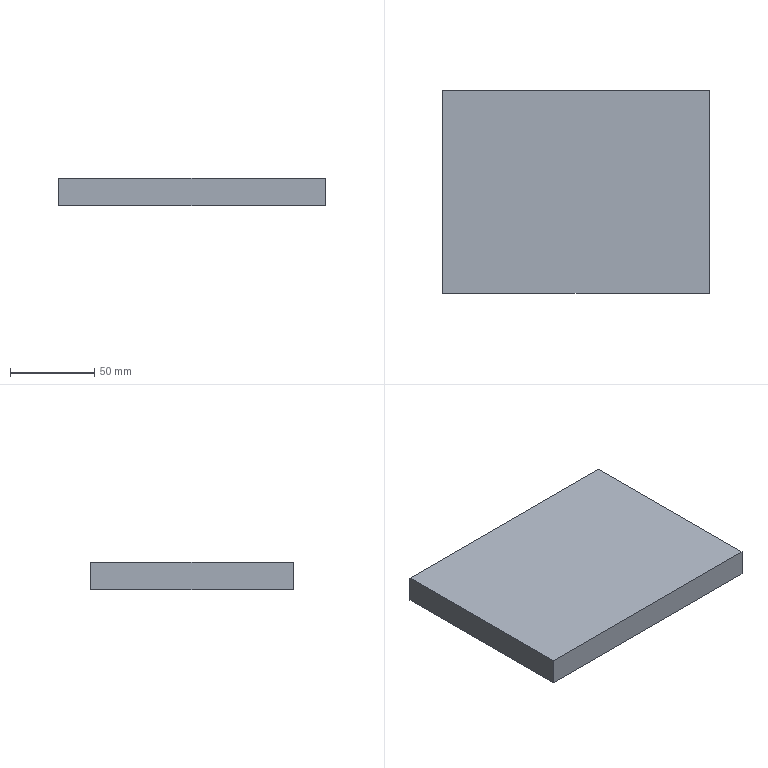Part | STEP file | 07-Square plate | 1 solid | 6 faces | box 158 x 120 x 16 mm | volume 303360 mm3 | plane 6
STEP:
#1=CARTESIAN_POINT('',(0.,0.,0.));
#2=DIRECTION('',(0.,0.,1.));
#3=DIRECTION('',(1.,0.,0.));
#4=AXIS2_PLACEMENT_3D('',#1,#2,#3);
#5=CARTESIAN_POINT('',(0.,0.,0.));
#6=VERTEX_POINT('',#5);
#7=CARTESIAN_POINT('',(0.,-120.,0.));
#8=VERTEX_POINT('',#7);
#9=CARTESIAN_POINT('',(0.,0.,0.));
#10=DIRECTION('',(0.,-1.,0.));
#11=VECTOR('',#10,1.);
#12=LINE('',#9,#11);
#13=CARTESIAN_POINT('',(0.,0.,16.));
#14=DIRECTION('',(1.,0.,0.));
#15=DIRECTION('',(0.,1.,0.));
#16=AXIS2_PLACEMENT_3D('',#13,#14,#15);
#17=PLANE('',#16);
#18=CARTESIAN_POINT('',(0.,-16.));
#19=DIRECTION('',(-1.,0.));
#20=VECTOR('',#19,1.);
#21=LINE('',#18,#20);
#22=(GEOMETRIC_REPRESENTATION_CONTEXT(2)PARAMETRIC_REPRESENTATION_CONTEXT()REPRESENTATION_CONTEXT('',''));
#23=DEFINITIONAL_REPRESENTATION('',(#21),#22);
#24=PCURVE('',#17,#23);
#25=CARTESIAN_POINT('',(0.,0.,0.));
#26=DIRECTION('',(0.,0.,1.));
#27=DIRECTION('',(1.,0.,0.));
#28=AXIS2_PLACEMENT_3D('',#25,#26,#27);
#29=PLANE('',#28);
#30=CARTESIAN_POINT('',(0.,0.));
#31=DIRECTION('',(0.,-1.));
#32=VECTOR('',#31,1.);
#33=LINE('',#30,#32);
#34=(GEOMETRIC_REPRESENTATION_CONTEXT(2)PARAMETRIC_REPRESENTATION_CONTEXT()REPRESENTATION_CONTEXT('',''));
#35=DEFINITIONAL_REPRESENTATION('',(#33),#34);
#36=PCURVE('',#29,#35);
#37=SURFACE_CURVE('',#12,(#24,#36),.PCURVE_S1.);
#38=EDGE_CURVE('',#6,#8,#37,.T.);
#39=ORIENTED_EDGE('',*,*,#38,.T.);
#40=CARTESIAN_POINT('',(0.,-120.,16.));
#41=VERTEX_POINT('',#40);
#42=CARTESIAN_POINT('',(0.,-120.,16.));
#43=DIRECTION('',(0.,0.,-1.));
#44=VECTOR('',#43,1.);
#45=LINE('',#42,#44);
#46=CARTESIAN_POINT('',(-120.,0.));
#47=DIRECTION('',(0.,-1.));
#48=VECTOR('',#47,1.);
#49=LINE('',#46,#48);
#50=(GEOMETRIC_REPRESENTATION_CONTEXT(2)PARAMETRIC_REPRESENTATION_CONTEXT()REPRESENTATION_CONTEXT('',''));
#51=DEFINITIONAL_REPRESENTATION('',(#49),#50);
#52=PCURVE('',#17,#51);
#53=CARTESIAN_POINT('',(0.,-120.,16.));
#54=DIRECTION('',(0.,1.,0.));
#55=DIRECTION('',(0.,0.,1.));
#56=AXIS2_PLACEMENT_3D('',#53,#54,#55);
#57=PLANE('',#56);
#58=CARTESIAN_POINT('',(0.,0.));
#59=DIRECTION('',(-1.,0.));
#60=VECTOR('',#59,1.);
#61=LINE('',#58,#60);
#62=(GEOMETRIC_REPRESENTATION_CONTEXT(2)PARAMETRIC_REPRESENTATION_CONTEXT()REPRESENTATION_CONTEXT('',''));
#63=DEFINITIONAL_REPRESENTATION('',(#61),#62);
#64=PCURVE('',#57,#63);
#65=SURFACE_CURVE('',#45,(#52,#64),.PCURVE_S1.);
#66=EDGE_CURVE('',#41,#8,#65,.T.);
#67=ORIENTED_EDGE('',*,*,#66,.F.);
#68=CARTESIAN_POINT('',(0.,0.,16.));
#69=VERTEX_POINT('',#68);
#70=CARTESIAN_POINT('',(0.,0.,16.));
#71=DIRECTION('',(0.,-1.,0.));
#72=VECTOR('',#71,1.);
#73=LINE('',#70,#72);
#74=CARTESIAN_POINT('',(0.,0.));
#75=DIRECTION('',(-1.,0.));
#76=VECTOR('',#75,1.);
#77=LINE('',#74,#76);
#78=(GEOMETRIC_REPRESENTATION_CONTEXT(2)PARAMETRIC_REPRESENTATION_CONTEXT()REPRESENTATION_CONTEXT('',''));
#79=DEFINITIONAL_REPRESENTATION('',(#77),#78);
#80=PCURVE('',#17,#79);
#81=CARTESIAN_POINT('',(0.,0.,16.));
#82=DIRECTION('',(0.,0.,1.));
#83=DIRECTION('',(1.,0.,0.));
#84=AXIS2_PLACEMENT_3D('',#81,#82,#83);
#85=PLANE('',#84);
#86=CARTESIAN_POINT('',(0.,0.));
#87=DIRECTION('',(0.,-1.));
#88=VECTOR('',#87,1.);
#89=LINE('',#86,#88);
#90=(GEOMETRIC_REPRESENTATION_CONTEXT(2)PARAMETRIC_REPRESENTATION_CONTEXT()REPRESENTATION_CONTEXT('',''));
#91=DEFINITIONAL_REPRESENTATION('',(#89),#90);
#92=PCURVE('',#85,#91);
#93=SURFACE_CURVE('',#73,(#80,#92),.PCURVE_S1.);
#94=EDGE_CURVE('',#69,#41,#93,.T.);
#95=ORIENTED_EDGE('',*,*,#94,.F.);
#96=CARTESIAN_POINT('',(0.,0.,16.));
#97=DIRECTION('',(0.,0.,-1.));
#98=VECTOR('',#97,1.);
#99=LINE('',#96,#98);
#100=CARTESIAN_POINT('',(0.,0.));
#101=DIRECTION('',(0.,-1.));
#102=VECTOR('',#101,1.);
#103=LINE('',#100,#102);
#104=(GEOMETRIC_REPRESENTATION_CONTEXT(2)PARAMETRIC_REPRESENTATION_CONTEXT()REPRESENTATION_CONTEXT('',''));
#105=DEFINITIONAL_REPRESENTATION('',(#103),#104);
#106=PCURVE('',#17,#105);
#107=CARTESIAN_POINT('',(0.,0.,16.));
#108=DIRECTION('',(0.,-1.,0.));
#109=DIRECTION('',(0.,0.,-1.));
#110=AXIS2_PLACEMENT_3D('',#107,#108,#109);
#111=PLANE('',#110);
#112=CARTESIAN_POINT('',(0.,0.));
#113=DIRECTION('',(1.,0.));
#114=VECTOR('',#113,1.);
#115=LINE('',#112,#114);
#116=(GEOMETRIC_REPRESENTATION_CONTEXT(2)PARAMETRIC_REPRESENTATION_CONTEXT()REPRESENTATION_CONTEXT('',''));
#117=DEFINITIONAL_REPRESENTATION('',(#115),#116);
#118=PCURVE('',#111,#117);
#119=SURFACE_CURVE('',#99,(#106,#118),.PCURVE_S1.);
#120=EDGE_CURVE('',#69,#6,#119,.T.);
#121=ORIENTED_EDGE('',*,*,#120,.T.);
#122=EDGE_LOOP('',(#39,#67,#95,#121));
#123=FACE_BOUND('',#122,.T.);
#124=ADVANCED_FACE('',(#123),#17,.F.);
#125=CARTESIAN_POINT('',(158.,-120.,0.));
#126=VERTEX_POINT('',#125);
#127=CARTESIAN_POINT('',(0.,-120.,0.));
#128=DIRECTION('',(1.,0.,0.));
#129=VECTOR('',#128,1.);
#130=LINE('',#127,#129);
#131=CARTESIAN_POINT('',(-16.,0.));
#132=DIRECTION('',(0.,1.));
#133=VECTOR('',#132,1.);
#134=LINE('',#131,#133);
#135=(GEOMETRIC_REPRESENTATION_CONTEXT(2)PARAMETRIC_REPRESENTATION_CONTEXT()REPRESENTATION_CONTEXT('',''));
#136=DEFINITIONAL_REPRESENTATION('',(#134),#135);
#137=PCURVE('',#57,#136);
#138=CARTESIAN_POINT('',(0.,-120.));
#139=DIRECTION('',(1.,0.));
#140=VECTOR('',#139,1.);
#141=LINE('',#138,#140);
#142=(GEOMETRIC_REPRESENTATION_CONTEXT(2)PARAMETRIC_REPRESENTATION_CONTEXT()REPRESENTATION_CONTEXT('',''));
#143=DEFINITIONAL_REPRESENTATION('',(#141),#142);
#144=PCURVE('',#29,#143);
#145=SURFACE_CURVE('',#130,(#137,#144),.PCURVE_S1.);
#146=EDGE_CURVE('',#8,#126,#145,.T.);
#147=ORIENTED_EDGE('',*,*,#146,.T.);
#148=CARTESIAN_POINT('',(158.,-120.,16.));
#149=VERTEX_POINT('',#148);
#150=CARTESIAN_POINT('',(158.,-120.,16.));
#151=DIRECTION('',(0.,0.,-1.));
#152=VECTOR('',#151,1.);
#153=LINE('',#150,#152);
#154=CARTESIAN_POINT('',(0.,158.));
#155=DIRECTION('',(-1.,0.));
#156=VECTOR('',#155,1.);
#157=LINE('',#154,#156);
#158=(GEOMETRIC_REPRESENTATION_CONTEXT(2)PARAMETRIC_REPRESENTATION_CONTEXT()REPRESENTATION_CONTEXT('',''));
#159=DEFINITIONAL_REPRESENTATION('',(#157),#158);
#160=PCURVE('',#57,#159);
#161=CARTESIAN_POINT('',(158.,0.,16.));
#162=DIRECTION('',(-1.,0.,0.));
#163=DIRECTION('',(0.,-1.,0.));
#164=AXIS2_PLACEMENT_3D('',#161,#162,#163);
#165=PLANE('',#164);
#166=CARTESIAN_POINT('',(120.,0.));
#167=DIRECTION('',(0.,-1.));
#168=VECTOR('',#167,1.);
#169=LINE('',#166,#168);
#170=(GEOMETRIC_REPRESENTATION_CONTEXT(2)PARAMETRIC_REPRESENTATION_CONTEXT()REPRESENTATION_CONTEXT('',''));
#171=DEFINITIONAL_REPRESENTATION('',(#169),#170);
#172=PCURVE('',#165,#171);
#173=SURFACE_CURVE('',#153,(#160,#172),.PCURVE_S1.);
#174=EDGE_CURVE('',#149,#126,#173,.T.);
#175=ORIENTED_EDGE('',*,*,#174,.F.);
#176=CARTESIAN_POINT('',(0.,-120.,16.));
#177=DIRECTION('',(1.,0.,0.));
#178=VECTOR('',#177,1.);
#179=LINE('',#176,#178);
#180=CARTESIAN_POINT('',(0.,0.));
#181=DIRECTION('',(0.,1.));
#182=VECTOR('',#181,1.);
#183=LINE('',#180,#182);
#184=(GEOMETRIC_REPRESENTATION_CONTEXT(2)PARAMETRIC_REPRESENTATION_CONTEXT()REPRESENTATION_CONTEXT('',''));
#185=DEFINITIONAL_REPRESENTATION('',(#183),#184);
#186=PCURVE('',#57,#185);
#187=CARTESIAN_POINT('',(0.,-120.));
#188=DIRECTION('',(1.,0.));
#189=VECTOR('',#188,1.);
#190=LINE('',#187,#189);
#191=(GEOMETRIC_REPRESENTATION_CONTEXT(2)PARAMETRIC_REPRESENTATION_CONTEXT()REPRESENTATION_CONTEXT('',''));
#192=DEFINITIONAL_REPRESENTATION('',(#190),#191);
#193=PCURVE('',#85,#192);
#194=SURFACE_CURVE('',#179,(#186,#193),.PCURVE_S1.);
#195=EDGE_CURVE('',#41,#149,#194,.T.);
#196=ORIENTED_EDGE('',*,*,#195,.F.);
#197=ORIENTED_EDGE('',*,*,#66,.T.);
#198=EDGE_LOOP('',(#147,#175,#196,#197));
#199=FACE_BOUND('',#198,.T.);
#200=ADVANCED_FACE('',(#199),#57,.F.);
#201=CARTESIAN_POINT('',(158.,0.,0.));
#202=VERTEX_POINT('',#201);
#203=CARTESIAN_POINT('',(158.,0.,0.));
#204=DIRECTION('',(0.,1.,0.));
#205=VECTOR('',#204,1.);
#206=LINE('',#203,#205);
#207=CARTESIAN_POINT('',(0.,-16.));
#208=DIRECTION('',(-1.,0.));
#209=VECTOR('',#208,1.);
#210=LINE('',#207,#209);
#211=(GEOMETRIC_REPRESENTATION_CONTEXT(2)PARAMETRIC_REPRESENTATION_CONTEXT()REPRESENTATION_CONTEXT('',''));
#212=DEFINITIONAL_REPRESENTATION('',(#210),#211);
#213=PCURVE('',#165,#212);
#214=CARTESIAN_POINT('',(158.,0.));
#215=DIRECTION('',(0.,1.));
#216=VECTOR('',#215,1.);
#217=LINE('',#214,#216);
#218=(GEOMETRIC_REPRESENTATION_CONTEXT(2)PARAMETRIC_REPRESENTATION_CONTEXT()REPRESENTATION_CONTEXT('',''));
#219=DEFINITIONAL_REPRESENTATION('',(#217),#218);
#220=PCURVE('',#29,#219);
#221=SURFACE_CURVE('',#206,(#213,#220),.PCURVE_S1.);
#222=EDGE_CURVE('',#126,#202,#221,.T.);
#223=ORIENTED_EDGE('',*,*,#222,.T.);
#224=CARTESIAN_POINT('',(158.,0.,16.));
#225=VERTEX_POINT('',#224);
#226=CARTESIAN_POINT('',(158.,0.,16.));
#227=DIRECTION('',(0.,0.,-1.));
#228=VECTOR('',#227,1.);
#229=LINE('',#226,#228);
#230=CARTESIAN_POINT('',(0.,0.));
#231=DIRECTION('',(0.,-1.));
#232=VECTOR('',#231,1.);
#233=LINE('',#230,#232);
#234=(GEOMETRIC_REPRESENTATION_CONTEXT(2)PARAMETRIC_REPRESENTATION_CONTEXT()REPRESENTATION_CONTEXT('',''));
#235=DEFINITIONAL_REPRESENTATION('',(#233),#234);
#236=PCURVE('',#165,#235);
#237=CARTESIAN_POINT('',(0.,158.));
#238=DIRECTION('',(1.,0.));
#239=VECTOR('',#238,1.);
#240=LINE('',#237,#239);
#241=(GEOMETRIC_REPRESENTATION_CONTEXT(2)PARAMETRIC_REPRESENTATION_CONTEXT()REPRESENTATION_CONTEXT('',''));
#242=DEFINITIONAL_REPRESENTATION('',(#240),#241);
#243=PCURVE('',#111,#242);
#244=SURFACE_CURVE('',#229,(#236,#243),.PCURVE_S1.);
#245=EDGE_CURVE('',#225,#202,#244,.T.);
#246=ORIENTED_EDGE('',*,*,#245,.F.);
#247=CARTESIAN_POINT('',(158.,0.,16.));
#248=DIRECTION('',(0.,1.,0.));
#249=VECTOR('',#248,1.);
#250=LINE('',#247,#249);
#251=CARTESIAN_POINT('',(0.,0.));
#252=DIRECTION('',(-1.,0.));
#253=VECTOR('',#252,1.);
#254=LINE('',#251,#253);
#255=(GEOMETRIC_REPRESENTATION_CONTEXT(2)PARAMETRIC_REPRESENTATION_CONTEXT()REPRESENTATION_CONTEXT('',''));
#256=DEFINITIONAL_REPRESENTATION('',(#254),#255);
#257=PCURVE('',#165,#256);
#258=CARTESIAN_POINT('',(158.,0.));
#259=DIRECTION('',(0.,1.));
#260=VECTOR('',#259,1.);
#261=LINE('',#258,#260);
#262=(GEOMETRIC_REPRESENTATION_CONTEXT(2)PARAMETRIC_REPRESENTATION_CONTEXT()REPRESENTATION_CONTEXT('',''));
#263=DEFINITIONAL_REPRESENTATION('',(#261),#262);
#264=PCURVE('',#85,#263);
#265=SURFACE_CURVE('',#250,(#257,#264),.PCURVE_S1.);
#266=EDGE_CURVE('',#149,#225,#265,.T.);
#267=ORIENTED_EDGE('',*,*,#266,.F.);
#268=ORIENTED_EDGE('',*,*,#174,.T.);
#269=EDGE_LOOP('',(#223,#246,#267,#268));
#270=FACE_BOUND('',#269,.T.);
#271=ADVANCED_FACE('',(#270),#165,.F.);
#272=CARTESIAN_POINT('',(0.,0.,0.));
#273=DIRECTION('',(-1.,0.,0.));
#274=VECTOR('',#273,1.);
#275=LINE('',#272,#274);
#276=CARTESIAN_POINT('',(16.,0.));
#277=DIRECTION('',(0.,-1.));
#278=VECTOR('',#277,1.);
#279=LINE('',#276,#278);
#280=(GEOMETRIC_REPRESENTATION_CONTEXT(2)PARAMETRIC_REPRESENTATION_CONTEXT()REPRESENTATION_CONTEXT('',''));
#281=DEFINITIONAL_REPRESENTATION('',(#279),#280);
#282=PCURVE('',#111,#281);
#283=CARTESIAN_POINT('',(0.,0.));
#284=DIRECTION('',(-1.,0.));
#285=VECTOR('',#284,1.);
#286=LINE('',#283,#285);
#287=(GEOMETRIC_REPRESENTATION_CONTEXT(2)PARAMETRIC_REPRESENTATION_CONTEXT()REPRESENTATION_CONTEXT('',''));
#288=DEFINITIONAL_REPRESENTATION('',(#286),#287);
#289=PCURVE('',#29,#288);
#290=SURFACE_CURVE('',#275,(#282,#289),.PCURVE_S1.);
#291=EDGE_CURVE('',#202,#6,#290,.T.);
#292=ORIENTED_EDGE('',*,*,#291,.T.);
#293=ORIENTED_EDGE('',*,*,#120,.F.);
#294=CARTESIAN_POINT('',(0.,0.,16.));
#295=DIRECTION('',(-1.,0.,0.));
#296=VECTOR('',#295,1.);
#297=LINE('',#294,#296);
#298=CARTESIAN_POINT('',(0.,0.));
#299=DIRECTION('',(0.,-1.));
#300=VECTOR('',#299,1.);
#301=LINE('',#298,#300);
#302=(GEOMETRIC_REPRESENTATION_CONTEXT(2)PARAMETRIC_REPRESENTATION_CONTEXT()REPRESENTATION_CONTEXT('',''));
#303=DEFINITIONAL_REPRESENTATION('',(#301),#302);
#304=PCURVE('',#111,#303);
#305=CARTESIAN_POINT('',(0.,0.));
#306=DIRECTION('',(-1.,0.));
#307=VECTOR('',#306,1.);
#308=LINE('',#305,#307);
#309=(GEOMETRIC_REPRESENTATION_CONTEXT(2)PARAMETRIC_REPRESENTATION_CONTEXT()REPRESENTATION_CONTEXT('',''));
#310=DEFINITIONAL_REPRESENTATION('',(#308),#309);
#311=PCURVE('',#85,#310);
#312=SURFACE_CURVE('',#297,(#304,#311),.PCURVE_S1.);
#313=EDGE_CURVE('',#225,#69,#312,.T.);
#314=ORIENTED_EDGE('',*,*,#313,.F.);
#315=ORIENTED_EDGE('',*,*,#245,.T.);
#316=EDGE_LOOP('',(#292,#293,#314,#315));
#317=FACE_BOUND('',#316,.T.);
#318=ADVANCED_FACE('',(#317),#111,.F.);
#319=ORIENTED_EDGE('',*,*,#94,.T.);
#320=ORIENTED_EDGE('',*,*,#195,.T.);
#321=ORIENTED_EDGE('',*,*,#266,.T.);
#322=ORIENTED_EDGE('',*,*,#313,.T.);
#323=EDGE_LOOP('',(#319,#320,#321,#322));
#324=FACE_BOUND('',#323,.T.);
#325=ADVANCED_FACE('',(#324),#85,.T.);
#326=ORIENTED_EDGE('',*,*,#38,.F.);
#327=ORIENTED_EDGE('',*,*,#291,.F.);
#328=ORIENTED_EDGE('',*,*,#222,.F.);
#329=ORIENTED_EDGE('',*,*,#146,.F.);
#330=EDGE_LOOP('',(#326,#327,#328,#329));
#331=FACE_BOUND('',#330,.T.);
#332=ADVANCED_FACE('',(#331),#29,.F.);
#333=CLOSED_SHELL('',(#124,#200,#271,#318,#325,#332));
#334=MANIFOLD_SOLID_BREP('',#333);
#335=(LENGTH_UNIT()NAMED_UNIT(*)SI_UNIT(.MILLI.,.METRE.));
#336=UNCERTAINTY_MEASURE_WITH_UNIT(LENGTH_MEASURE(0.0000001),#335,'','');
#337=(NAMED_UNIT(*)PLANE_ANGLE_UNIT()SI_UNIT($,.RADIAN.));
#338=(NAMED_UNIT(*)SI_UNIT($,.STERADIAN.)SOLID_ANGLE_UNIT());
#339=(GEOMETRIC_REPRESENTATION_CONTEXT(3)GLOBAL_UNCERTAINTY_ASSIGNED_CONTEXT((#336))GLOBAL_UNIT_ASSIGNED_CONTEXT((#335,#337,#338))REPRESENTATION_CONTEXT('',''));
#340=ADVANCED_BREP_SHAPE_REPRESENTATION('',(#4,#334),#339);